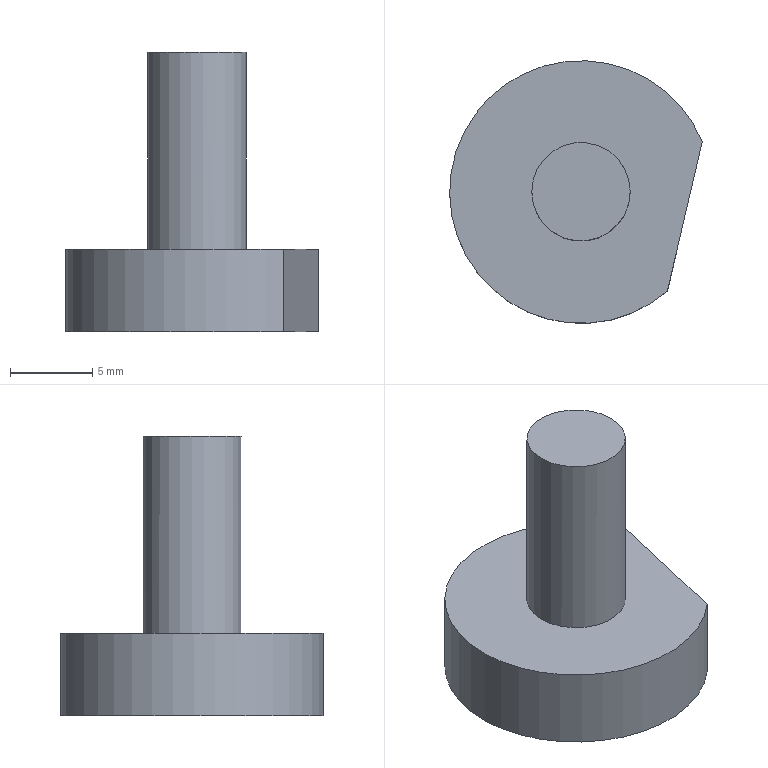Part | NX | features solid 2 | 1 solid | 6 faces | box 15.392 x 16 x 17 mm | volume 1297 mm3 | plane 4 | cylinder 2 | commonest cylinder face diameters 6 x1 16 x1
STEP:
#1=CARTESIAN_POINT('',(725.16,-171.735,141.));
#2=VERTEX_POINT('',#1);
#3=CARTESIAN_POINT('',(728.16,-171.735,141.));
#4=DIRECTION('',(0.,0.,-1.));
#5=DIRECTION('',(-1.,0.,0.));
#6=AXIS2_PLACEMENT_3D('',#3,#4,#5);
#7=CIRCLE('',#6,3.);
#8=EDGE_CURVE('',#2,#2,#7,.T.);
#9=ORIENTED_EDGE('',*,*,#8,.T.);
#10=EDGE_LOOP('',(#9));
#11=FACE_BOUND('',#10,.T.);
#12=CARTESIAN_POINT('',(733.426,-177.757,141.));
#13=VERTEX_POINT('',#12);
#14=CARTESIAN_POINT('',(735.551,-168.675,141.));
#15=VERTEX_POINT('',#14);
#16=CARTESIAN_POINT('',(734.489,-173.216,141.));
#17=DIRECTION('',(0.2278,0.9737,0.));
#18=VECTOR('',#17,1000.);
#19=LINE('',#16,#18);
#20=EDGE_CURVE('',#13,#15,#19,.T.);
#21=ORIENTED_EDGE('',*,*,#20,.T.);
#22=CARTESIAN_POINT('',(728.16,-171.735,141.));
#23=DIRECTION('',(0.,0.,1.));
#24=DIRECTION('',(0.9737,-0.2278,0.));
#25=AXIS2_PLACEMENT_3D('',#22,#23,#24);
#26=CIRCLE('',#25,8.);
#27=EDGE_CURVE('',#15,#13,#26,.T.);
#28=ORIENTED_EDGE('',*,*,#27,.T.);
#29=EDGE_LOOP('',(#21,#28));
#30=FACE_BOUND('',#29,.T.);
#31=CARTESIAN_POINT('',(728.16,-171.735,141.));
#32=DIRECTION('',(0.,0.,1.));
#33=DIRECTION('',(-0.9737,0.2278,0.));
#34=AXIS2_PLACEMENT_3D('',#31,#32,#33);
#35=PLANE('',#34);
#36=ADVANCED_FACE('',(#11,#30),#35,.T.);
#37=CARTESIAN_POINT('',(733.426,-177.757,136.));
#38=VERTEX_POINT('',#37);
#39=CARTESIAN_POINT('',(735.551,-168.675,136.));
#40=VERTEX_POINT('',#39);
#41=CARTESIAN_POINT('',(744.399,-130.86,136.));
#42=DIRECTION('',(0.2278,0.9737,0.));
#43=VECTOR('',#42,1000.);
#44=LINE('',#41,#43);
#45=EDGE_CURVE('',#38,#40,#44,.T.);
#46=ORIENTED_EDGE('',*,*,#45,.F.);
#47=CARTESIAN_POINT('',(728.16,-171.735,136.));
#48=DIRECTION('',(0.,0.,-1.));
#49=DIRECTION('',(-0.9737,0.2278,0.));
#50=AXIS2_PLACEMENT_3D('',#47,#48,#49);
#51=CIRCLE('',#50,8.);
#52=EDGE_CURVE('',#38,#40,#51,.T.);
#53=ORIENTED_EDGE('',*,*,#52,.T.);
#54=EDGE_LOOP('',(#46,#53));
#55=FACE_BOUND('',#54,.T.);
#56=CARTESIAN_POINT('',(728.16,-171.735,136.));
#57=DIRECTION('',(0.,0.,-1.));
#58=DIRECTION('',(0.9737,-0.2278,0.));
#59=AXIS2_PLACEMENT_3D('',#56,#57,#58);
#60=PLANE('',#59);
#61=ADVANCED_FACE('',(#55),#60,.T.);
#62=CARTESIAN_POINT('',(735.551,-168.675,136.));
#63=DIRECTION('',(0.,0.,1.));
#64=VECTOR('',#63,1000.);
#65=LINE('',#62,#64);
#66=EDGE_CURVE('',#15,#40,#65,.F.);
#67=ORIENTED_EDGE('',*,*,#66,.T.);
#68=ORIENTED_EDGE('',*,*,#52,.F.);
#69=CARTESIAN_POINT('',(733.426,-177.757,136.));
#70=DIRECTION('',(0.,0.,1.));
#71=VECTOR('',#70,1000.);
#72=LINE('',#69,#71);
#73=EDGE_CURVE('',#38,#13,#72,.T.);
#74=ORIENTED_EDGE('',*,*,#73,.T.);
#75=ORIENTED_EDGE('',*,*,#27,.F.);
#76=EDGE_LOOP('',(#67,#68,#74,#75));
#77=FACE_BOUND('',#76,.T.);
#78=CARTESIAN_POINT('',(728.16,-171.735,136.));
#79=DIRECTION('',(0.,0.,1.));
#80=DIRECTION('',(-0.9737,0.2278,0.));
#81=AXIS2_PLACEMENT_3D('',#78,#79,#80);
#82=CYLINDRICAL_SURFACE('',#81,8.);
#83=ADVANCED_FACE('',(#77),#82,.T.);
#84=ORIENTED_EDGE('',*,*,#66,.F.);
#85=ORIENTED_EDGE('',*,*,#20,.F.);
#86=ORIENTED_EDGE('',*,*,#73,.F.);
#87=ORIENTED_EDGE('',*,*,#45,.T.);
#88=EDGE_LOOP('',(#84,#85,#86,#87));
#89=FACE_BOUND('',#88,.T.);
#90=CARTESIAN_POINT('',(744.399,-130.86,136.));
#91=DIRECTION('',(-0.9737,0.2278,0.));
#92=DIRECTION('',(0.,0.,-1.));
#93=AXIS2_PLACEMENT_3D('',#90,#91,#92);
#94=PLANE('',#93);
#95=ADVANCED_FACE('',(#89),#94,.F.);
#96=CARTESIAN_POINT('',(731.081,-172.419,153.));
#97=VERTEX_POINT('',#96);
#98=CARTESIAN_POINT('',(728.16,-171.735,153.));
#99=DIRECTION('',(0.,0.,1.));
#100=DIRECTION('',(0.9737,-0.2278,0.));
#101=AXIS2_PLACEMENT_3D('',#98,#99,#100);
#102=CIRCLE('',#101,3.);
#103=EDGE_CURVE('',#97,#97,#102,.T.);
#104=ORIENTED_EDGE('',*,*,#103,.T.);
#105=EDGE_LOOP('',(#104));
#106=FACE_BOUND('',#105,.T.);
#107=CARTESIAN_POINT('',(728.16,-171.735,153.));
#108=DIRECTION('',(0.,0.,1.));
#109=DIRECTION('',(-0.9737,0.2278,0.));
#110=AXIS2_PLACEMENT_3D('',#107,#108,#109);
#111=PLANE('',#110);
#112=ADVANCED_FACE('',(#106),#111,.T.);
#113=ORIENTED_EDGE('',*,*,#103,.F.);
#114=EDGE_LOOP('',(#113));
#115=FACE_BOUND('',#114,.T.);
#116=ORIENTED_EDGE('',*,*,#8,.F.);
#117=EDGE_LOOP('',(#116));
#118=FACE_BOUND('',#117,.T.);
#119=CARTESIAN_POINT('',(728.16,-171.735,141.));
#120=DIRECTION('',(0.,0.,1.));
#121=DIRECTION('',(-0.9737,0.2278,0.));
#122=AXIS2_PLACEMENT_3D('',#119,#120,#121);
#123=CYLINDRICAL_SURFACE('',#122,3.);
#124=ADVANCED_FACE('',(#115,#118),#123,.T.);
#125=CLOSED_SHELL('',(#36,#61,#83,#95,#112,#124));
#126=MANIFOLD_SOLID_BREP('',#125);
#127=(LENGTH_UNIT()NAMED_UNIT(*)SI_UNIT(.MILLI.,.METRE.));
#128=UNCERTAINTY_MEASURE_WITH_UNIT(LENGTH_MEASURE(0.00001),#127,'','');
#129=(NAMED_UNIT(*)PLANE_ANGLE_UNIT()SI_UNIT($,.RADIAN.));
#130=(NAMED_UNIT(*)SI_UNIT($,.STERADIAN.)SOLID_ANGLE_UNIT());
#131=(GEOMETRIC_REPRESENTATION_CONTEXT(3)GLOBAL_UNCERTAINTY_ASSIGNED_CONTEXT((#128))GLOBAL_UNIT_ASSIGNED_CONTEXT((#127,#129,#130))REPRESENTATION_CONTEXT('',''));
#132=ADVANCED_BREP_SHAPE_REPRESENTATION('',(#126),#131);